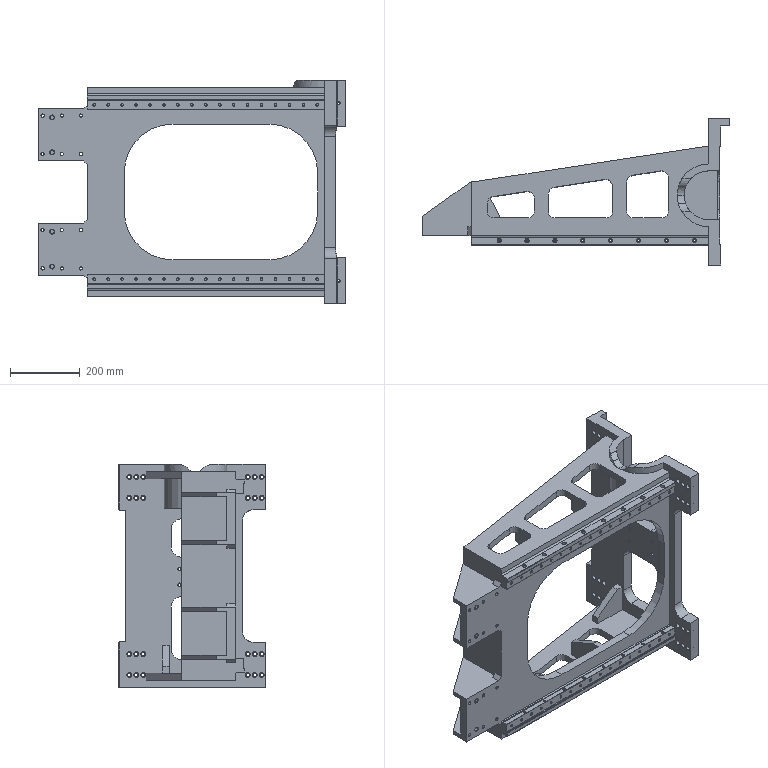Part | SolidWorks | features BaseBody 1 | 1 solid | 927 faces | box 881 x 420 x 640 mm | volume 19459611 mm3 | cone 336 | cylinder 325 | plane 266 | commonest cylinder face diameters 6.5 x104 9 x48 13.5 x48 8.5 x32 11 x32 40 x24